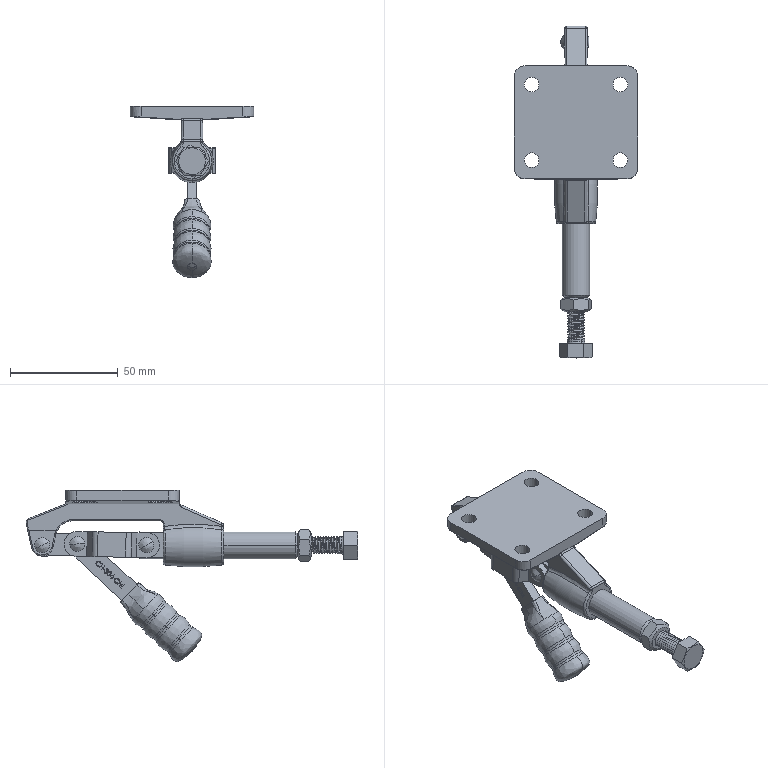Part | SolidWorks | features BaseBody 11 | 11 solids | 795 faces | box 57.2 x 153.749 x 79.304 mm | volume 52807 mm3 | cylinder 266 | plane 247 | spline 216 | torus 37 | cone 27 | sphere 2 | commonest cylinder face diameters 6.8 x77 8 x76 4 x25 1 x12 6.5 x12 6 x8